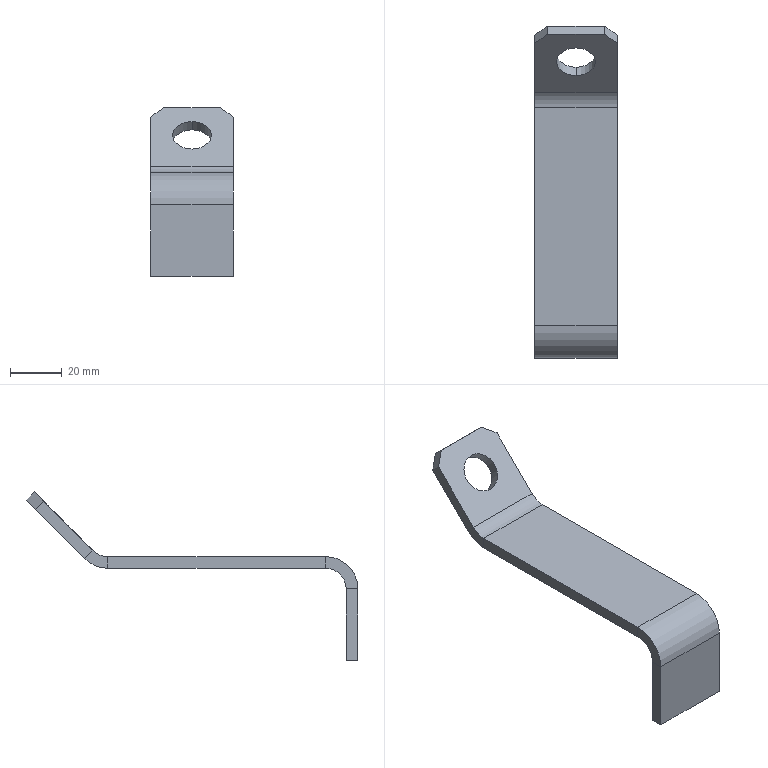Part | SolidWorks | features Chamfer 1, FlatPattern 1, ICE 1, SMBaseFlange 1, SheetMetal 1 | 1 solid | 26 faces | box 32 x 128.182 x 65 mm | volume 23267 mm3 | plane 20 | cylinder 6 | commonest cylinder face diameters 15 x2 16 x2 25 x2
STEP:
#1=CARTESIAN_POINT('',(0.,109.09,49.09));
#2=VERTEX_POINT('',#1);
#3=CARTESIAN_POINT('',(0.,119.697,59.697));
#4=VERTEX_POINT('',#3);
#5=CARTESIAN_POINT('',(0.,114.393,54.393));
#6=DIRECTION('',(0.,0.7071,-0.7071));
#7=DIRECTION('',(0.,-0.7071,-0.7071));
#8=AXIS2_PLACEMENT_3D('',#5,#6,#7);
#9=CIRCLE('',#8,7.5);
#10=EDGE_CURVE('',#2,#4,#9,.T.);
#11=ORIENTED_EDGE('',*,*,#10,.F.);
#12=CARTESIAN_POINT('',(0.,112.272,45.908));
#13=VERTEX_POINT('',#12);
#14=CARTESIAN_POINT('',(0.,46.589,111.591));
#15=DIRECTION('',(0.,0.7071,-0.7071));
#16=VECTOR('',#15,1000.);
#17=LINE('',#14,#16);
#18=EDGE_CURVE('',#2,#13,#17,.T.);
#19=ORIENTED_EDGE('',*,*,#18,.T.);
#20=CARTESIAN_POINT('',(0.,122.879,56.515));
#21=VERTEX_POINT('',#20);
#22=CARTESIAN_POINT('',(0.,117.575,51.211));
#23=DIRECTION('',(0.,0.7071,-0.7071));
#24=DIRECTION('',(0.,0.7071,0.7071));
#25=AXIS2_PLACEMENT_3D('',#22,#23,#24);
#26=CIRCLE('',#25,7.5);
#27=EDGE_CURVE('',#13,#21,#26,.T.);
#28=ORIENTED_EDGE('',*,*,#27,.T.);
#29=CARTESIAN_POINT('',(0.,57.196,122.198));
#30=DIRECTION('',(0.,0.7071,-0.7071));
#31=VECTOR('',#30,1000.);
#32=LINE('',#29,#31);
#33=EDGE_CURVE('',#4,#21,#32,.T.);
#34=ORIENTED_EDGE('',*,*,#33,.F.);
#35=EDGE_LOOP('',(#11,#19,#28,#34));
#36=FACE_OUTER_BOUND('',#35,.T.);
#37=CARTESIAN_POINT('',(0.,51.892,116.894));
#38=DIRECTION('',(0.,0.7071,-0.7071));
#39=DIRECTION('',(0.,0.7071,0.7071));
#40=AXIS2_PLACEMENT_3D('',#37,#38,#39);
#41=CYLINDRICAL_SURFACE('',#40,7.5);
#42=ADVANCED_FACE('',(#36),#41,.F.);
#43=CARTESIAN_POINT('',(16.,12.5,40.));
#44=VERTEX_POINT('',#43);
#45=CARTESIAN_POINT('',(16.,12.5,35.5));
#46=VERTEX_POINT('',#45);
#47=CARTESIAN_POINT('',(16.,12.5,40.));
#48=DIRECTION('',(0.,0.,-1.));
#49=VECTOR('',#48,1000.);
#50=LINE('',#47,#49);
#51=EDGE_CURVE('',#44,#46,#50,.T.);
#52=ORIENTED_EDGE('',*,*,#51,.F.);
#53=CARTESIAN_POINT('',(16.,0.,27.5));
#54=VERTEX_POINT('',#53);
#55=CARTESIAN_POINT('',(16.,12.5,27.5));
#56=DIRECTION('',(-1.,0.,0.));
#57=DIRECTION('',(0.,0.,-1.));
#58=AXIS2_PLACEMENT_3D('',#55,#56,#57);
#59=CIRCLE('',#58,12.5);
#60=EDGE_CURVE('',#54,#44,#59,.T.);
#61=ORIENTED_EDGE('',*,*,#60,.F.);
#62=CARTESIAN_POINT('',(16.,4.5,27.5));
#63=VERTEX_POINT('',#62);
#64=CARTESIAN_POINT('',(16.,4.5,27.5));
#65=DIRECTION('',(0.,-1.,0.));
#66=VECTOR('',#65,1000.);
#67=LINE('',#64,#66);
#68=EDGE_CURVE('',#63,#54,#67,.T.);
#69=ORIENTED_EDGE('',*,*,#68,.F.);
#70=CARTESIAN_POINT('',(16.,12.5,27.5));
#71=DIRECTION('',(-1.,0.,0.));
#72=DIRECTION('',(0.,0.,-1.));
#73=AXIS2_PLACEMENT_3D('',#70,#71,#72);
#74=CIRCLE('',#73,8.);
#75=EDGE_CURVE('',#63,#46,#74,.T.);
#76=ORIENTED_EDGE('',*,*,#75,.T.);
#77=EDGE_LOOP('',(#52,#61,#69,#76));
#78=FACE_OUTER_BOUND('',#77,.T.);
#79=CARTESIAN_POINT('',(16.,12.5,40.));
#80=DIRECTION('',(1.,0.,0.));
#81=DIRECTION('',(0.,0.,-1.));
#82=AXIS2_PLACEMENT_3D('',#79,#80,#81);
#83=PLANE('',#82);
#84=ADVANCED_FACE('',(#78),#83,.T.);
#85=CARTESIAN_POINT('',(16.,96.686,40.));
#86=VERTEX_POINT('',#85);
#87=CARTESIAN_POINT('',(16.,0.,40.));
#88=DIRECTION('',(0.,1.,0.));
#89=VECTOR('',#88,1000.);
#90=LINE('',#87,#89);
#91=EDGE_CURVE('',#44,#86,#90,.T.);
#92=ORIENTED_EDGE('',*,*,#91,.F.);
#93=ORIENTED_EDGE('',*,*,#51,.T.);
#94=CARTESIAN_POINT('',(16.,96.686,35.5));
#95=VERTEX_POINT('',#94);
#96=CARTESIAN_POINT('',(16.,0.,35.5));
#97=DIRECTION('',(0.,1.,0.));
#98=VECTOR('',#97,1000.);
#99=LINE('',#96,#98);
#100=EDGE_CURVE('',#46,#95,#99,.T.);
#101=ORIENTED_EDGE('',*,*,#100,.T.);
#102=CARTESIAN_POINT('',(16.,96.686,35.5));
#103=DIRECTION('',(0.,0.,1.));
#104=VECTOR('',#103,1000.);
#105=LINE('',#102,#104);
#106=EDGE_CURVE('',#95,#86,#105,.T.);
#107=ORIENTED_EDGE('',*,*,#106,.T.);
#108=EDGE_LOOP('',(#92,#93,#101,#107));
#109=FACE_OUTER_BOUND('',#108,.T.);
#110=CARTESIAN_POINT('',(16.,4.5,27.5));
#111=DIRECTION('',(1.,0.,0.));
#112=DIRECTION('',(0.,0.,-1.));
#113=AXIS2_PLACEMENT_3D('',#110,#111,#112);
#114=PLANE('',#113);
#115=ADVANCED_FACE('',(#109),#114,.T.);
#116=CARTESIAN_POINT('',(-16.,0.,27.5));
#117=VERTEX_POINT('',#116);
#118=CARTESIAN_POINT('',(-16.,4.5,27.5));
#119=VERTEX_POINT('',#118);
#120=CARTESIAN_POINT('',(-16.,0.,27.5));
#121=DIRECTION('',(0.,1.,0.));
#122=VECTOR('',#121,1000.);
#123=LINE('',#120,#122);
#124=EDGE_CURVE('',#117,#119,#123,.T.);
#125=ORIENTED_EDGE('',*,*,#124,.F.);
#126=CARTESIAN_POINT('',(-16.,12.5,40.));
#127=VERTEX_POINT('',#126);
#128=CARTESIAN_POINT('',(-16.,12.5,27.5));
#129=DIRECTION('',(-1.,0.,0.));
#130=DIRECTION('',(0.,0.,-1.));
#131=AXIS2_PLACEMENT_3D('',#128,#129,#130);
#132=CIRCLE('',#131,12.5);
#133=EDGE_CURVE('',#117,#127,#132,.T.);
#134=ORIENTED_EDGE('',*,*,#133,.T.);
#135=CARTESIAN_POINT('',(-16.,12.5,35.5));
#136=VERTEX_POINT('',#135);
#137=CARTESIAN_POINT('',(-16.,12.5,35.5));
#138=DIRECTION('',(0.,0.,1.));
#139=VECTOR('',#138,1000.);
#140=LINE('',#137,#139);
#141=EDGE_CURVE('',#136,#127,#140,.T.);
#142=ORIENTED_EDGE('',*,*,#141,.F.);
#143=CARTESIAN_POINT('',(-16.,12.5,27.5));
#144=DIRECTION('',(-1.,0.,0.));
#145=DIRECTION('',(0.,0.,-1.));
#146=AXIS2_PLACEMENT_3D('',#143,#144,#145);
#147=CIRCLE('',#146,8.);
#148=EDGE_CURVE('',#119,#136,#147,.T.);
#149=ORIENTED_EDGE('',*,*,#148,.F.);
#150=EDGE_LOOP('',(#125,#134,#142,#149));
#151=FACE_OUTER_BOUND('',#150,.T.);
#152=CARTESIAN_POINT('',(-16.,0.,27.5));
#153=DIRECTION('',(-1.,0.,0.));
#154=DIRECTION('',(0.,0.,1.));
#155=AXIS2_PLACEMENT_3D('',#152,#153,#154);
#156=PLANE('',#155);
#157=ADVANCED_FACE('',(#151),#156,.T.);
#158=CARTESIAN_POINT('',(-16.,0.,0.));
#159=VERTEX_POINT('',#158);
#160=CARTESIAN_POINT('',(-16.,0.,0.));
#161=DIRECTION('',(0.,0.,1.));
#162=VECTOR('',#161,1000.);
#163=LINE('',#160,#162);
#164=EDGE_CURVE('',#159,#117,#163,.T.);
#165=ORIENTED_EDGE('',*,*,#164,.T.);
#166=ORIENTED_EDGE('',*,*,#124,.T.);
#167=CARTESIAN_POINT('',(-16.,4.5,0.));
#168=VERTEX_POINT('',#167);
#169=CARTESIAN_POINT('',(-16.,4.5,0.));
#170=DIRECTION('',(0.,0.,1.));
#171=VECTOR('',#170,1000.);
#172=LINE('',#169,#171);
#173=EDGE_CURVE('',#168,#119,#172,.T.);
#174=ORIENTED_EDGE('',*,*,#173,.F.);
#175=CARTESIAN_POINT('',(-16.,4.5,0.));
#176=DIRECTION('',(0.,-1.,0.));
#177=VECTOR('',#176,1000.);
#178=LINE('',#175,#177);
#179=EDGE_CURVE('',#168,#159,#178,.T.);
#180=ORIENTED_EDGE('',*,*,#179,.T.);
#181=EDGE_LOOP('',(#165,#166,#174,#180));
#182=FACE_OUTER_BOUND('',#181,.T.);
#183=CARTESIAN_POINT('',(-16.,12.5,35.5));
#184=DIRECTION('',(-1.,0.,0.));
#185=DIRECTION('',(0.,0.,1.));
#186=AXIS2_PLACEMENT_3D('',#183,#184,#185);
#187=PLANE('',#186);
#188=ADVANCED_FACE('',(#182),#187,.T.);
#189=CARTESIAN_POINT('',(16.,102.343,42.343));
#190=VERTEX_POINT('',#189);
#191=CARTESIAN_POINT('',(16.,105.525,39.161));
#192=VERTEX_POINT('',#191);
#193=CARTESIAN_POINT('',(16.,102.343,42.343));
#194=DIRECTION('',(0.,0.7071,-0.7071));
#195=VECTOR('',#194,1000.);
#196=LINE('',#193,#195);
#197=EDGE_CURVE('',#190,#192,#196,.T.);
#198=ORIENTED_EDGE('',*,*,#197,.F.);
#199=CARTESIAN_POINT('',(16.,96.686,48.));
#200=DIRECTION('',(1.,0.,0.));
#201=DIRECTION('',(0.,0.,1.));
#202=AXIS2_PLACEMENT_3D('',#199,#200,#201);
#203=CIRCLE('',#202,8.);
#204=EDGE_CURVE('',#86,#190,#203,.T.);
#205=ORIENTED_EDGE('',*,*,#204,.F.);
#206=ORIENTED_EDGE('',*,*,#106,.F.);
#207=CARTESIAN_POINT('',(16.,96.686,48.));
#208=DIRECTION('',(1.,0.,0.));
#209=DIRECTION('',(0.,0.,-1.));
#210=AXIS2_PLACEMENT_3D('',#207,#208,#209);
#211=CIRCLE('',#210,12.5);
#212=EDGE_CURVE('',#95,#192,#211,.T.);
#213=ORIENTED_EDGE('',*,*,#212,.T.);
#214=EDGE_LOOP('',(#198,#205,#206,#213));
#215=FACE_OUTER_BOUND('',#214,.T.);
#216=CARTESIAN_POINT('',(16.,102.343,42.343));
#217=DIRECTION('',(1.,0.,0.));
#218=DIRECTION('',(0.,0.,-1.));
#219=AXIS2_PLACEMENT_3D('',#216,#217,#218);
#220=PLANE('',#219);
#221=ADVANCED_FACE('',(#215),#220,.T.);
#222=CARTESIAN_POINT('',(16.,124.646,58.282));
#223=VERTEX_POINT('',#222);
#224=CARTESIAN_POINT('',(16.,103.182,36.818));
#225=DIRECTION('',(0.,0.7071,0.7071));
#226=VECTOR('',#225,1000.);
#227=LINE('',#224,#226);
#228=EDGE_CURVE('',#192,#223,#227,.T.);
#229=ORIENTED_EDGE('',*,*,#228,.T.);
#230=CARTESIAN_POINT('',(16.,121.464,61.464));
#231=VERTEX_POINT('',#230);
#232=CARTESIAN_POINT('',(16.,122.058,60.871));
#233=DIRECTION('',(0.,-0.7071,0.7071));
#234=VECTOR('',#233,1000.);
#235=LINE('',#232,#234);
#236=EDGE_CURVE('',#223,#231,#235,.T.);
#237=ORIENTED_EDGE('',*,*,#236,.T.);
#238=CARTESIAN_POINT('',(16.,100.,40.));
#239=DIRECTION('',(0.,0.7071,0.7071));
#240=VECTOR('',#239,1000.);
#241=LINE('',#238,#240);
#242=EDGE_CURVE('',#190,#231,#241,.T.);
#243=ORIENTED_EDGE('',*,*,#242,.F.);
#244=ORIENTED_EDGE('',*,*,#197,.T.);
#245=EDGE_LOOP('',(#229,#237,#243,#244));
#246=FACE_OUTER_BOUND('',#245,.T.);
#247=CARTESIAN_POINT('',(16.,96.686,35.5));
#248=DIRECTION('',(1.,0.,0.));
#249=DIRECTION('',(0.,0.,-1.));
#250=AXIS2_PLACEMENT_3D('',#247,#248,#249);
#251=PLANE('',#250);
#252=ADVANCED_FACE('',(#246),#251,.T.);
#253=CARTESIAN_POINT('',(-16.,96.686,40.));
#254=VERTEX_POINT('',#253);
#255=CARTESIAN_POINT('',(-16.,96.686,35.5));
#256=VERTEX_POINT('',#255);
#257=CARTESIAN_POINT('',(-16.,96.686,40.));
#258=DIRECTION('',(0.,0.,-1.));
#259=VECTOR('',#258,1000.);
#260=LINE('',#257,#259);
#261=EDGE_CURVE('',#254,#256,#260,.T.);
#262=ORIENTED_EDGE('',*,*,#261,.F.);
#263=CARTESIAN_POINT('',(-16.,102.343,42.343));
#264=VERTEX_POINT('',#263);
#265=CARTESIAN_POINT('',(-16.,96.686,48.));
#266=DIRECTION('',(1.,0.,0.));
#267=DIRECTION('',(0.,0.,1.));
#268=AXIS2_PLACEMENT_3D('',#265,#266,#267);
#269=CIRCLE('',#268,8.);
#270=EDGE_CURVE('',#254,#264,#269,.T.);
#271=ORIENTED_EDGE('',*,*,#270,.T.);
#272=CARTESIAN_POINT('',(-16.,105.525,39.161));
#273=VERTEX_POINT('',#272);
#274=CARTESIAN_POINT('',(-16.,105.525,39.161));
#275=DIRECTION('',(0.,-0.7071,0.7071));
#276=VECTOR('',#275,1000.);
#277=LINE('',#274,#276);
#278=EDGE_CURVE('',#273,#264,#277,.T.);
#279=ORIENTED_EDGE('',*,*,#278,.F.);
#280=CARTESIAN_POINT('',(-16.,96.686,48.));
#281=DIRECTION('',(1.,0.,0.));
#282=DIRECTION('',(0.,0.,-1.));
#283=AXIS2_PLACEMENT_3D('',#280,#281,#282);
#284=CIRCLE('',#283,12.5);
#285=EDGE_CURVE('',#256,#273,#284,.T.);
#286=ORIENTED_EDGE('',*,*,#285,.F.);
#287=EDGE_LOOP('',(#262,#271,#279,#286));
#288=FACE_OUTER_BOUND('',#287,.T.);
#289=CARTESIAN_POINT('',(-16.,96.686,40.));
#290=DIRECTION('',(-1.,0.,0.));
#291=DIRECTION('',(0.,0.,1.));
#292=AXIS2_PLACEMENT_3D('',#289,#290,#291);
#293=PLANE('',#292);
#294=ADVANCED_FACE('',(#288),#293,.T.);
#295=CARTESIAN_POINT('',(-16.,0.,40.));
#296=DIRECTION('',(0.,1.,0.));
#297=VECTOR('',#296,1000.);
#298=LINE('',#295,#297);
#299=EDGE_CURVE('',#127,#254,#298,.T.);
#300=ORIENTED_EDGE('',*,*,#299,.T.);
#301=ORIENTED_EDGE('',*,*,#261,.T.);
#302=CARTESIAN_POINT('',(-16.,0.,35.5));
#303=DIRECTION('',(0.,1.,0.));
#304=VECTOR('',#303,1000.);
#305=LINE('',#302,#304);
#306=EDGE_CURVE('',#136,#256,#305,.T.);
#307=ORIENTED_EDGE('',*,*,#306,.F.);
#308=ORIENTED_EDGE('',*,*,#141,.T.);
#309=EDGE_LOOP('',(#300,#301,#307,#308));
#310=FACE_OUTER_BOUND('',#309,.T.);
#311=CARTESIAN_POINT('',(-16.,105.525,39.161));
#312=DIRECTION('',(-1.,0.,0.));
#313=DIRECTION('',(0.,0.,1.));
#314=AXIS2_PLACEMENT_3D('',#311,#312,#313);
#315=PLANE('',#314);
#316=ADVANCED_FACE('',(#310),#315,.T.);
#317=CARTESIAN_POINT('',(0.,117.575,51.211));
#318=DIRECTION('',(0.,0.7071,-0.7071));
#319=DIRECTION('',(0.,0.7071,0.7071));
#320=AXIS2_PLACEMENT_3D('',#317,#318,#319);
#321=CIRCLE('',#320,7.5);
#322=EDGE_CURVE('',#21,#13,#321,.T.);
#323=ORIENTED_EDGE('',*,*,#322,.F.);
#324=ORIENTED_EDGE('',*,*,#27,.F.);
#325=EDGE_LOOP('',(#323,#324));
#326=FACE_BOUND('',#325,.T.);
#327=CARTESIAN_POINT('',(-16.,124.646,58.282));
#328=VERTEX_POINT('',#327);
#329=CARTESIAN_POINT('',(-16.,103.182,36.818));
#330=DIRECTION('',(0.,0.7071,0.7071));
#331=VECTOR('',#330,1000.);
#332=LINE('',#329,#331);
#333=EDGE_CURVE('',#273,#328,#332,.T.);
#334=ORIENTED_EDGE('',*,*,#333,.T.);
#335=CARTESIAN_POINT('',(-11.,128.182,61.818));
#336=VERTEX_POINT('',#335);
#337=CARTESIAN_POINT('',(-16.,124.646,58.282));
#338=DIRECTION('',(0.7071,0.5,0.5));
#339=VECTOR('',#338,1000.);
#340=LINE('',#337,#339);
#341=EDGE_CURVE('',#328,#336,#340,.T.);
#342=ORIENTED_EDGE('',*,*,#341,.T.);
#343=CARTESIAN_POINT('',(11.,128.182,61.818));
#344=VERTEX_POINT('',#343);
#345=CARTESIAN_POINT('',(16.,128.182,61.818));
#346=DIRECTION('',(-1.,0.,0.));
#347=VECTOR('',#346,1000.);
#348=LINE('',#345,#347);
#349=EDGE_CURVE('',#344,#336,#348,.T.);
#350=ORIENTED_EDGE('',*,*,#349,.F.);
#351=CARTESIAN_POINT('',(11.,128.182,61.818));
#352=DIRECTION('',(0.7071,-0.5,-0.5));
#353=VECTOR('',#352,1000.);
#354=LINE('',#351,#353);
#355=EDGE_CURVE('',#344,#223,#354,.T.);
#356=ORIENTED_EDGE('',*,*,#355,.T.);
#357=ORIENTED_EDGE('',*,*,#228,.F.);
#358=CARTESIAN_POINT('',(16.,105.525,39.161));
#359=DIRECTION('',(-1.,0.,0.));
#360=VECTOR('',#359,1000.);
#361=LINE('',#358,#360);
#362=EDGE_CURVE('',#192,#273,#361,.T.);
#363=ORIENTED_EDGE('',*,*,#362,.T.);
#364=EDGE_LOOP('',(#334,#342,#350,#356,#357,#363));
#365=FACE_OUTER_BOUND('',#364,.T.);
#366=CARTESIAN_POINT('',(16.,103.182,36.818));
#367=DIRECTION('',(0.,-0.7071,0.7071));
#368=DIRECTION('',(0.,-0.7071,-0.7071));
#369=AXIS2_PLACEMENT_3D('',#366,#367,#368);
#370=PLANE('',#369);
#371=ADVANCED_FACE('',(#326,#365),#370,.F.);
#372=ORIENTED_EDGE('',*,*,#349,.T.);
#373=CARTESIAN_POINT('',(-11.,125.,65.));
#374=VERTEX_POINT('',#373);
#375=CARTESIAN_POINT('',(-11.,125.,65.));
#376=DIRECTION('',(0.,-0.7071,0.7071));
#377=VECTOR('',#376,1000.);
#378=LINE('',#375,#377);
#379=EDGE_CURVE('',#336,#374,#378,.T.);
#380=ORIENTED_EDGE('',*,*,#379,.T.);
#381=CARTESIAN_POINT('',(11.,125.,65.));
#382=VERTEX_POINT('',#381);
#383=CARTESIAN_POINT('',(16.,125.,65.));
#384=DIRECTION('',(-1.,0.,0.));
#385=VECTOR('',#384,1000.);
#386=LINE('',#383,#385);
#387=EDGE_CURVE('',#382,#374,#386,.T.);
#388=ORIENTED_EDGE('',*,*,#387,.F.);
#389=CARTESIAN_POINT('',(11.,125.,65.));
#390=DIRECTION('',(0.,0.7071,-0.7071));
#391=VECTOR('',#390,1000.);
#392=LINE('',#389,#391);
#393=EDGE_CURVE('',#382,#344,#392,.T.);
#394=ORIENTED_EDGE('',*,*,#393,.T.);
#395=EDGE_LOOP('',(#372,#380,#388,#394));
#396=FACE_OUTER_BOUND('',#395,.T.);
#397=CARTESIAN_POINT('',(16.,125.,65.));
#398=DIRECTION('',(0.,0.7071,0.7071));
#399=DIRECTION('',(0.,-0.7071,0.7071));
#400=AXIS2_PLACEMENT_3D('',#397,#398,#399);
#401=PLANE('',#400);
#402=ADVANCED_FACE('',(#396),#401,.T.);
#403=CARTESIAN_POINT('',(0.,114.393,54.393));
#404=DIRECTION('',(0.,0.7071,-0.7071));
#405=DIRECTION('',(0.,-0.7071,-0.7071));
#406=AXIS2_PLACEMENT_3D('',#403,#404,#405);
#407=CIRCLE('',#406,7.5);
#408=EDGE_CURVE('',#4,#2,#407,.T.);
#409=ORIENTED_EDGE('',*,*,#408,.T.);
#410=ORIENTED_EDGE('',*,*,#10,.T.);
#411=EDGE_LOOP('',(#409,#410));
#412=FACE_BOUND('',#411,.T.);
#413=ORIENTED_EDGE('',*,*,#387,.T.);
#414=CARTESIAN_POINT('',(-16.,121.464,61.464));
#415=VERTEX_POINT('',#414);
#416=CARTESIAN_POINT('',(-15.178,122.046,62.046));
#417=DIRECTION('',(-0.7071,-0.5,-0.5));
#418=VECTOR('',#417,1000.);
#419=LINE('',#416,#418);
#420=EDGE_CURVE('',#374,#415,#419,.T.);
#421=ORIENTED_EDGE('',*,*,#420,.T.);
#422=CARTESIAN_POINT('',(-16.,100.,40.));
#423=DIRECTION('',(0.,0.7071,0.7071));
#424=VECTOR('',#423,1000.);
#425=LINE('',#422,#424);
#426=EDGE_CURVE('',#264,#415,#425,.T.);
#427=ORIENTED_EDGE('',*,*,#426,.F.);
#428=CARTESIAN_POINT('',(16.,102.343,42.343));
#429=DIRECTION('',(-1.,0.,0.));
#430=VECTOR('',#429,1000.);
#431=LINE('',#428,#430);
#432=EDGE_CURVE('',#190,#264,#431,.T.);
#433=ORIENTED_EDGE('',*,*,#432,.F.);
#434=ORIENTED_EDGE('',*,*,#242,.T.);
#435=CARTESIAN_POINT('',(31.178,110.732,50.732));
#436=DIRECTION('',(-0.7071,0.5,0.5));
#437=VECTOR('',#436,1000.);
#438=LINE('',#435,#437);
#439=EDGE_CURVE('',#231,#382,#438,.T.);
#440=ORIENTED_EDGE('',*,*,#439,.T.);
#441=EDGE_LOOP('',(#413,#421,#427,#433,#434,#440));
#442=FACE_OUTER_BOUND('',#441,.T.);
#443=CARTESIAN_POINT('',(16.,100.,40.));
#444=DIRECTION('',(0.,-0.7071,0.7071));
#445=DIRECTION('',(0.,-0.7071,-0.7071));
#446=AXIS2_PLACEMENT_3D('',#443,#444,#445);
#447=PLANE('',#446);
#448=ADVANCED_FACE('',(#412,#442),#447,.T.);
#449=ORIENTED_EDGE('',*,*,#270,.F.);
#450=CARTESIAN_POINT('',(16.,96.686,40.));
#451=DIRECTION('',(-1.,0.,0.));
#452=VECTOR('',#451,1000.);
#453=LINE('',#450,#452);
#454=EDGE_CURVE('',#86,#254,#453,.T.);
#455=ORIENTED_EDGE('',*,*,#454,.F.);
#456=ORIENTED_EDGE('',*,*,#204,.T.);
#457=ORIENTED_EDGE('',*,*,#432,.T.);
#458=EDGE_LOOP('',(#449,#455,#456,#457));
#459=FACE_OUTER_BOUND('',#458,.T.);
#460=CARTESIAN_POINT('',(16.,96.686,48.));
#461=DIRECTION('',(-1.,0.,0.));
#462=DIRECTION('',(0.,0.,1.));
#463=AXIS2_PLACEMENT_3D('',#460,#461,#462);
#464=CYLINDRICAL_SURFACE('',#463,8.);
#465=ADVANCED_FACE('',(#459),#464,.F.);
#466=ORIENTED_EDGE('',*,*,#299,.F.);
#467=CARTESIAN_POINT('',(16.,12.5,40.));
#468=DIRECTION('',(-1.,0.,0.));
#469=VECTOR('',#468,1000.);
#470=LINE('',#467,#469);
#471=EDGE_CURVE('',#44,#127,#470,.T.);
#472=ORIENTED_EDGE('',*,*,#471,.F.);
#473=ORIENTED_EDGE('',*,*,#91,.T.);
#474=ORIENTED_EDGE('',*,*,#454,.T.);
#475=EDGE_LOOP('',(#466,#472,#473,#474));
#476=FACE_OUTER_BOUND('',#475,.T.);
#477=CARTESIAN_POINT('',(16.,0.,40.));
#478=DIRECTION('',(0.,0.,1.));
#479=DIRECTION('',(1.,0.,0.));
#480=AXIS2_PLACEMENT_3D('',#477,#478,#479);
#481=PLANE('',#480);
#482=ADVANCED_FACE('',(#476),#481,.T.);
#483=ORIENTED_EDGE('',*,*,#133,.F.);
#484=CARTESIAN_POINT('',(16.,0.,27.5));
#485=DIRECTION('',(-1.,0.,0.));
#486=VECTOR('',#485,1000.);
#487=LINE('',#484,#486);
#488=EDGE_CURVE('',#54,#117,#487,.T.);
#489=ORIENTED_EDGE('',*,*,#488,.F.);
#490=ORIENTED_EDGE('',*,*,#60,.T.);
#491=ORIENTED_EDGE('',*,*,#471,.T.);
#492=EDGE_LOOP('',(#483,#489,#490,#491));
#493=FACE_OUTER_BOUND('',#492,.T.);
#494=CARTESIAN_POINT('',(16.,12.5,27.5));
#495=DIRECTION('',(-1.,0.,0.));
#496=DIRECTION('',(0.,0.,1.));
#497=AXIS2_PLACEMENT_3D('',#494,#495,#496);
#498=CYLINDRICAL_SURFACE('',#497,12.5);
#499=ADVANCED_FACE('',(#493),#498,.T.);
#500=ORIENTED_EDGE('',*,*,#164,.F.);
#501=CARTESIAN_POINT('',(16.,0.,0.));
#502=VERTEX_POINT('',#501);
#503=CARTESIAN_POINT('',(16.,0.,0.));
#504=DIRECTION('',(-1.,0.,0.));
#505=VECTOR('',#504,1000.);
#506=LINE('',#503,#505);
#507=EDGE_CURVE('',#502,#159,#506,.T.);
#508=ORIENTED_EDGE('',*,*,#507,.F.);
#509=CARTESIAN_POINT('',(16.,0.,0.));
#510=DIRECTION('',(0.,0.,1.));
#511=VECTOR('',#510,1000.);
#512=LINE('',#509,#511);
#513=EDGE_CURVE('',#502,#54,#512,.T.);
#514=ORIENTED_EDGE('',*,*,#513,.T.);
#515=ORIENTED_EDGE('',*,*,#488,.T.);
#516=EDGE_LOOP('',(#500,#508,#514,#515));
#517=FACE_OUTER_BOUND('',#516,.T.);
#518=CARTESIAN_POINT('',(16.,0.,0.));
#519=DIRECTION('',(0.,-1.,0.));
#520=DIRECTION('',(0.,0.,-1.));
#521=AXIS2_PLACEMENT_3D('',#518,#519,#520);
#522=PLANE('',#521);
#523=ADVANCED_FACE('',(#517),#522,.T.);
#524=ORIENTED_EDGE('',*,*,#179,.F.);
#525=CARTESIAN_POINT('',(16.,4.5,0.));
#526=VERTEX_POINT('',#525);
#527=CARTESIAN_POINT('',(16.,4.5,0.));
#528=DIRECTION('',(-1.,0.,0.));
#529=VECTOR('',#528,1000.);
#530=LINE('',#527,#529);
#531=EDGE_CURVE('',#526,#168,#530,.T.);
#532=ORIENTED_EDGE('',*,*,#531,.F.);
#533=CARTESIAN_POINT('',(16.,4.5,0.));
#534=DIRECTION('',(0.,-1.,0.));
#535=VECTOR('',#534,1000.);
#536=LINE('',#533,#535);
#537=EDGE_CURVE('',#526,#502,#536,.T.);
#538=ORIENTED_EDGE('',*,*,#537,.T.);
#539=ORIENTED_EDGE('',*,*,#507,.T.);
#540=EDGE_LOOP('',(#524,#532,#538,#539));
#541=FACE_OUTER_BOUND('',#540,.T.);
#542=CARTESIAN_POINT('',(16.,4.5,0.));
#543=DIRECTION('',(0.,0.,-1.));
#544=DIRECTION('',(-1.,0.,0.));
#545=AXIS2_PLACEMENT_3D('',#542,#543,#544);
#546=PLANE('',#545);
#547=ADVANCED_FACE('',(#541),#546,.T.);
#548=ORIENTED_EDGE('',*,*,#173,.T.);
#549=CARTESIAN_POINT('',(16.,4.5,27.5));
#550=DIRECTION('',(-1.,0.,0.));
#551=VECTOR('',#550,1000.);
#552=LINE('',#549,#551);
#553=EDGE_CURVE('',#63,#119,#552,.T.);
#554=ORIENTED_EDGE('',*,*,#553,.F.);
#555=CARTESIAN_POINT('',(16.,4.5,0.));
#556=DIRECTION('',(0.,0.,1.));
#557=VECTOR('',#556,1000.);
#558=LINE('',#555,#557);
#559=EDGE_CURVE('',#526,#63,#558,.T.);
#560=ORIENTED_EDGE('',*,*,#559,.F.);
#561=ORIENTED_EDGE('',*,*,#531,.T.);
#562=EDGE_LOOP('',(#548,#554,#560,#561));
#563=FACE_OUTER_BOUND('',#562,.T.);
#564=CARTESIAN_POINT('',(16.,4.5,0.));
#565=DIRECTION('',(0.,-1.,0.));
#566=DIRECTION('',(0.,0.,-1.));
#567=AXIS2_PLACEMENT_3D('',#564,#565,#566);
#568=PLANE('',#567);
#569=ADVANCED_FACE('',(#563),#568,.F.);
#570=ORIENTED_EDGE('',*,*,#148,.T.);
#571=CARTESIAN_POINT('',(16.,12.5,35.5));
#572=DIRECTION('',(-1.,0.,0.));
#573=VECTOR('',#572,1000.);
#574=LINE('',#571,#573);
#575=EDGE_CURVE('',#46,#136,#574,.T.);
#576=ORIENTED_EDGE('',*,*,#575,.F.);
#577=ORIENTED_EDGE('',*,*,#75,.F.);
#578=ORIENTED_EDGE('',*,*,#553,.T.);
#579=EDGE_LOOP('',(#570,#576,#577,#578));
#580=FACE_OUTER_BOUND('',#579,.T.);
#581=CARTESIAN_POINT('',(16.,12.5,27.5));
#582=DIRECTION('',(-1.,0.,0.));
#583=DIRECTION('',(0.,0.,1.));
#584=AXIS2_PLACEMENT_3D('',#581,#582,#583);
#585=CYLINDRICAL_SURFACE('',#584,8.);
#586=ADVANCED_FACE('',(#580),#585,.F.);
#587=ORIENTED_EDGE('',*,*,#306,.T.);
#588=CARTESIAN_POINT('',(16.,96.686,35.5));
#589=DIRECTION('',(-1.,0.,0.));
#590=VECTOR('',#589,1000.);
#591=LINE('',#588,#590);
#592=EDGE_CURVE('',#95,#256,#591,.T.);
#593=ORIENTED_EDGE('',*,*,#592,.F.);
#594=ORIENTED_EDGE('',*,*,#100,.F.);
#595=ORIENTED_EDGE('',*,*,#575,.T.);
#596=EDGE_LOOP('',(#587,#593,#594,#595));
#597=FACE_OUTER_BOUND('',#596,.T.);
#598=CARTESIAN_POINT('',(16.,0.,35.5));
#599=DIRECTION('',(0.,0.,1.));
#600=DIRECTION('',(1.,0.,0.));
#601=AXIS2_PLACEMENT_3D('',#598,#599,#600);
#602=PLANE('',#601);
#603=ADVANCED_FACE('',(#597),#602,.F.);
#604=ORIENTED_EDGE('',*,*,#285,.T.);
#605=ORIENTED_EDGE('',*,*,#362,.F.);
#606=ORIENTED_EDGE('',*,*,#212,.F.);
#607=ORIENTED_EDGE('',*,*,#592,.T.);
#608=EDGE_LOOP('',(#604,#605,#606,#607));
#609=FACE_OUTER_BOUND('',#608,.T.);
#610=CARTESIAN_POINT('',(16.,96.686,48.));
#611=DIRECTION('',(-1.,0.,0.));
#612=DIRECTION('',(0.,0.,1.));
#613=AXIS2_PLACEMENT_3D('',#610,#611,#612);
#614=CYLINDRICAL_SURFACE('',#613,12.5);
#615=ADVANCED_FACE('',(#609),#614,.T.);
#616=ORIENTED_EDGE('',*,*,#559,.T.);
#617=ORIENTED_EDGE('',*,*,#68,.T.);
#618=ORIENTED_EDGE('',*,*,#513,.F.);
#619=ORIENTED_EDGE('',*,*,#537,.F.);
#620=EDGE_LOOP('',(#616,#617,#618,#619));
#621=FACE_OUTER_BOUND('',#620,.T.);
#622=CARTESIAN_POINT('',(16.,96.686,48.));
#623=DIRECTION('',(-1.,0.,0.));
#624=DIRECTION('',(0.,0.,1.));
#625=AXIS2_PLACEMENT_3D('',#622,#623,#624);
#626=PLANE('',#625);
#627=ADVANCED_FACE('',(#621),#626,.F.);
#628=ORIENTED_EDGE('',*,*,#426,.T.);
#629=CARTESIAN_POINT('',(-16.,115.808,67.121));
#630=DIRECTION('',(0.,0.7071,-0.7071));
#631=VECTOR('',#630,1000.);
#632=LINE('',#629,#631);
#633=EDGE_CURVE('',#415,#328,#632,.T.);
#634=ORIENTED_EDGE('',*,*,#633,.T.);
#635=ORIENTED_EDGE('',*,*,#333,.F.);
#636=ORIENTED_EDGE('',*,*,#278,.T.);
#637=EDGE_LOOP('',(#628,#634,#635,#636));
#638=FACE_OUTER_BOUND('',#637,.T.);
#639=CARTESIAN_POINT('',(-16.,96.686,48.));
#640=DIRECTION('',(-1.,0.,0.));
#641=DIRECTION('',(0.,0.,1.));
#642=AXIS2_PLACEMENT_3D('',#639,#640,#641);
#643=PLANE('',#642);
#644=ADVANCED_FACE('',(#638),#643,.T.);
#645=ORIENTED_EDGE('',*,*,#18,.F.);
#646=ORIENTED_EDGE('',*,*,#408,.F.);
#647=ORIENTED_EDGE('',*,*,#33,.T.);
#648=ORIENTED_EDGE('',*,*,#322,.T.);
#649=EDGE_LOOP('',(#645,#646,#647,#648));
#650=FACE_OUTER_BOUND('',#649,.T.);
#651=CARTESIAN_POINT('',(0.,51.892,116.894));
#652=DIRECTION('',(0.,0.7071,-0.7071));
#653=DIRECTION('',(0.,0.7071,0.7071));
#654=AXIS2_PLACEMENT_3D('',#651,#652,#653);
#655=CYLINDRICAL_SURFACE('',#654,7.5);
#656=ADVANCED_FACE('',(#650),#655,.F.);
#657=ORIENTED_EDGE('',*,*,#420,.F.);
#658=ORIENTED_EDGE('',*,*,#379,.F.);
#659=ORIENTED_EDGE('',*,*,#341,.F.);
#660=ORIENTED_EDGE('',*,*,#633,.F.);
#661=EDGE_LOOP('',(#657,#658,#659,#660));
#662=FACE_OUTER_BOUND('',#661,.T.);
#663=CARTESIAN_POINT('',(-16.,115.808,67.121));
#664=DIRECTION('',(0.7071,-0.5,-0.5));
#665=DIRECTION('',(0.,0.7071,-0.7071));
#666=AXIS2_PLACEMENT_3D('',#663,#664,#665);
#667=PLANE('',#666);
#668=ADVANCED_FACE('',(#662),#667,.F.);
#669=ORIENTED_EDGE('',*,*,#439,.F.);
#670=ORIENTED_EDGE('',*,*,#236,.F.);
#671=ORIENTED_EDGE('',*,*,#355,.F.);
#672=ORIENTED_EDGE('',*,*,#393,.F.);
#673=EDGE_LOOP('',(#669,#670,#671,#672));
#674=FACE_OUTER_BOUND('',#673,.T.);
#675=CARTESIAN_POINT('',(11.,125.,65.));
#676=DIRECTION('',(-0.7071,-0.5,-0.5));
#677=DIRECTION('',(0.,0.7071,-0.7071));
#678=AXIS2_PLACEMENT_3D('',#675,#676,#677);
#679=PLANE('',#678);
#680=ADVANCED_FACE('',(#674),#679,.F.);
#681=CLOSED_SHELL('',(#42,#84,#115,#157,#188,#221,#252,#294,#316,#371,#402,#448,#465,#482,#499,#523,#547,#569,#586,#603,#615,#627,#644,#656,#668,#680));
#682=MANIFOLD_SOLID_BREP('',#681);
#683=CARTESIAN_POINT('',(0.,0.,0.));
#684=DIRECTION('',(0.,0.,1.));
#685=DIRECTION('',(1.,0.,0.));
#686=AXIS2_PLACEMENT_3D('',#683,#684,#685);
#687=(LENGTH_UNIT()NAMED_UNIT(*)SI_UNIT(.MILLI.,.METRE.));
#688=UNCERTAINTY_MEASURE_WITH_UNIT(LENGTH_MEASURE(0.00001),#687,'','');
#689=(NAMED_UNIT(*)PLANE_ANGLE_UNIT()SI_UNIT($,.RADIAN.));
#690=(NAMED_UNIT(*)SI_UNIT($,.STERADIAN.)SOLID_ANGLE_UNIT());
#691=(GEOMETRIC_REPRESENTATION_CONTEXT(3)GLOBAL_UNCERTAINTY_ASSIGNED_CONTEXT((#688))GLOBAL_UNIT_ASSIGNED_CONTEXT((#687,#689,#690))REPRESENTATION_CONTEXT('',''));
#692=ADVANCED_BREP_SHAPE_REPRESENTATION('',(#682,#686),#691);